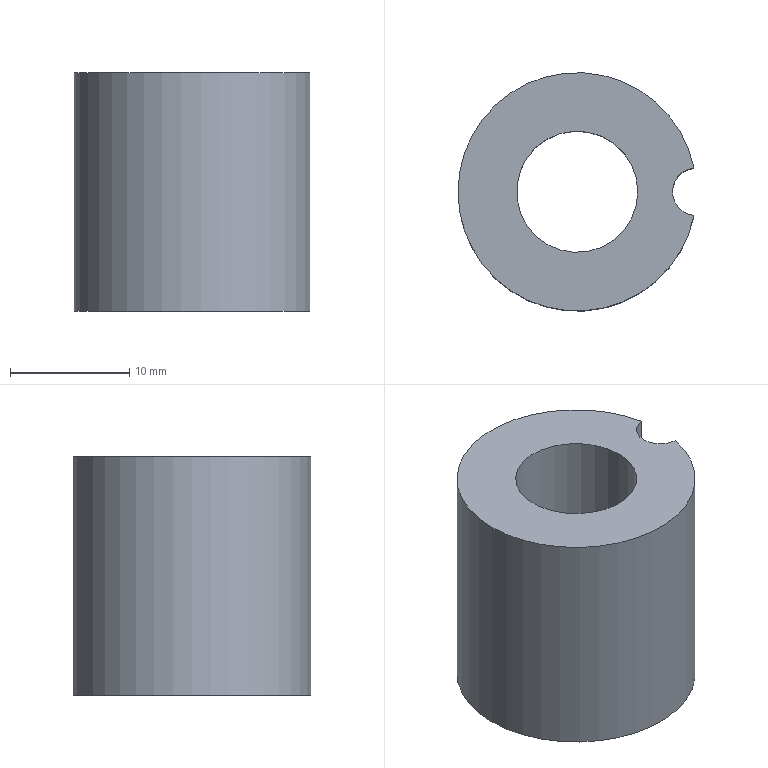Part | NX | features solid 2 | 1 solid | 7 faces | box 19.8 x 20 x 20 mm | volume 4017 mm3 | cylinder 4 | plane 3 | commonest cylinder face diameters 4 x1 10.17 x1 12.6 x1 20 x1
STEP:
#1=CARTESIAN_POINT('',(-210.056,-19.136,32.703));
#2=VERTEX_POINT('',#1);
#3=CARTESIAN_POINT('',(-210.056,-15.156,32.703));
#4=VERTEX_POINT('',#3);
#5=CARTESIAN_POINT('',(-209.856,-17.146,32.703));
#6=DIRECTION('',(0.,0.,-1.));
#7=DIRECTION('',(-1.,0.,0.));
#8=AXIS2_PLACEMENT_3D('',#5,#6,#7);
#9=CIRCLE('',#8,2.);
#10=EDGE_CURVE('',#2,#4,#9,.T.);
#11=ORIENTED_EDGE('',*,*,#10,.T.);
#12=CARTESIAN_POINT('',(-219.856,-17.146,32.703));
#13=DIRECTION('',(0.,0.,-1.));
#14=DIRECTION('',(-1.,0.,0.));
#15=AXIS2_PLACEMENT_3D('',#12,#13,#14);
#16=CIRCLE('',#15,10.);
#17=EDGE_CURVE('',#2,#4,#16,.T.);
#18=ORIENTED_EDGE('',*,*,#17,.F.);
#19=EDGE_LOOP('',(#11,#18));
#20=FACE_BOUND('',#19,.T.);
#21=CARTESIAN_POINT('',(-214.771,-17.146,32.703));
#22=VERTEX_POINT('',#21);
#23=CARTESIAN_POINT('',(-219.856,-17.146,32.703));
#24=DIRECTION('',(0.,0.,1.));
#25=DIRECTION('',(1.,0.,0.));
#26=AXIS2_PLACEMENT_3D('',#23,#24,#25);
#27=CIRCLE('',#26,5.085);
#28=EDGE_CURVE('',#22,#22,#27,.F.);
#29=ORIENTED_EDGE('',*,*,#28,.T.);
#30=EDGE_LOOP('',(#29));
#31=FACE_BOUND('',#30,.T.);
#32=CARTESIAN_POINT('',(-219.856,-17.146,32.703));
#33=DIRECTION('',(0.,0.,1.));
#34=DIRECTION('',(1.,0.,0.));
#35=AXIS2_PLACEMENT_3D('',#32,#33,#34);
#36=PLANE('',#35);
#37=ADVANCED_FACE('',(#20,#31),#36,.T.);
#38=CARTESIAN_POINT('',(-210.056,-15.156,12.703));
#39=VERTEX_POINT('',#38);
#40=CARTESIAN_POINT('',(-210.056,-19.136,12.703));
#41=VERTEX_POINT('',#40);
#42=CARTESIAN_POINT('',(-209.856,-17.146,12.703));
#43=DIRECTION('',(0.,0.,1.));
#44=DIRECTION('',(1.,0.,0.));
#45=AXIS2_PLACEMENT_3D('',#42,#43,#44);
#46=CIRCLE('',#45,2.);
#47=EDGE_CURVE('',#39,#41,#46,.T.);
#48=ORIENTED_EDGE('',*,*,#47,.T.);
#49=CARTESIAN_POINT('',(-219.856,-17.146,12.703));
#50=DIRECTION('',(0.,0.,1.));
#51=DIRECTION('',(1.,0.,0.));
#52=AXIS2_PLACEMENT_3D('',#49,#50,#51);
#53=CIRCLE('',#52,10.);
#54=EDGE_CURVE('',#39,#41,#53,.T.);
#55=ORIENTED_EDGE('',*,*,#54,.F.);
#56=EDGE_LOOP('',(#48,#55));
#57=FACE_BOUND('',#56,.T.);
#58=CARTESIAN_POINT('',(-213.556,-17.146,12.703));
#59=VERTEX_POINT('',#58);
#60=CARTESIAN_POINT('',(-219.856,-17.146,12.703));
#61=DIRECTION('',(0.,0.,1.));
#62=DIRECTION('',(1.,0.,0.));
#63=AXIS2_PLACEMENT_3D('',#60,#61,#62);
#64=CIRCLE('',#63,6.3);
#65=EDGE_CURVE('',#59,#59,#64,.T.);
#66=ORIENTED_EDGE('',*,*,#65,.T.);
#67=EDGE_LOOP('',(#66));
#68=FACE_BOUND('',#67,.T.);
#69=CARTESIAN_POINT('',(-219.856,-17.146,12.703));
#70=DIRECTION('',(0.,0.,-1.));
#71=DIRECTION('',(-1.,0.,0.));
#72=AXIS2_PLACEMENT_3D('',#69,#70,#71);
#73=PLANE('',#72);
#74=ADVANCED_FACE('',(#57,#68),#73,.T.);
#75=CARTESIAN_POINT('',(-210.056,-15.156,22.703));
#76=DIRECTION('',(0.,0.,1.));
#77=VECTOR('',#76,1000.);
#78=LINE('',#75,#77);
#79=EDGE_CURVE('',#39,#4,#78,.T.);
#80=ORIENTED_EDGE('',*,*,#79,.F.);
#81=ORIENTED_EDGE('',*,*,#54,.T.);
#82=CARTESIAN_POINT('',(-210.056,-19.136,22.703));
#83=DIRECTION('',(0.,0.,1.));
#84=VECTOR('',#83,1000.);
#85=LINE('',#82,#84);
#86=EDGE_CURVE('',#2,#41,#85,.F.);
#87=ORIENTED_EDGE('',*,*,#86,.F.);
#88=ORIENTED_EDGE('',*,*,#17,.T.);
#89=EDGE_LOOP('',(#80,#81,#87,#88));
#90=FACE_BOUND('',#89,.T.);
#91=CARTESIAN_POINT('',(-219.856,-17.146,12.703));
#92=DIRECTION('',(0.,0.,1.));
#93=DIRECTION('',(1.,0.,0.));
#94=AXIS2_PLACEMENT_3D('',#91,#92,#93);
#95=CYLINDRICAL_SURFACE('',#94,10.);
#96=ADVANCED_FACE('',(#90),#95,.T.);
#97=CARTESIAN_POINT('',(-214.771,-17.146,24.703));
#98=VERTEX_POINT('',#97);
#99=CARTESIAN_POINT('',(-219.856,-17.146,24.703));
#100=DIRECTION('',(0.,0.,1.));
#101=DIRECTION('',(1.,0.,0.));
#102=AXIS2_PLACEMENT_3D('',#99,#100,#101);
#103=CIRCLE('',#102,5.085);
#104=EDGE_CURVE('',#98,#98,#103,.T.);
#105=ORIENTED_EDGE('',*,*,#104,.T.);
#106=EDGE_LOOP('',(#105));
#107=FACE_BOUND('',#106,.T.);
#108=CARTESIAN_POINT('',(-226.156,-17.146,24.703));
#109=VERTEX_POINT('',#108);
#110=CARTESIAN_POINT('',(-219.856,-17.146,24.703));
#111=DIRECTION('',(0.,0.,-1.));
#112=DIRECTION('',(-1.,0.,0.));
#113=AXIS2_PLACEMENT_3D('',#110,#111,#112);
#114=CIRCLE('',#113,6.3);
#115=EDGE_CURVE('',#109,#109,#114,.T.);
#116=ORIENTED_EDGE('',*,*,#115,.T.);
#117=EDGE_LOOP('',(#116));
#118=FACE_BOUND('',#117,.T.);
#119=CARTESIAN_POINT('',(-219.856,-17.146,24.703));
#120=DIRECTION('',(0.,0.,1.));
#121=DIRECTION('',(1.,0.,0.));
#122=AXIS2_PLACEMENT_3D('',#119,#120,#121);
#123=PLANE('',#122);
#124=ADVANCED_FACE('',(#107,#118),#123,.F.);
#125=ORIENTED_EDGE('',*,*,#115,.F.);
#126=EDGE_LOOP('',(#125));
#127=FACE_BOUND('',#126,.T.);
#128=ORIENTED_EDGE('',*,*,#65,.F.);
#129=EDGE_LOOP('',(#128));
#130=FACE_BOUND('',#129,.T.);
#131=CARTESIAN_POINT('',(-219.856,-17.146,12.703));
#132=DIRECTION('',(0.,0.,1.));
#133=DIRECTION('',(1.,0.,0.));
#134=AXIS2_PLACEMENT_3D('',#131,#132,#133);
#135=CYLINDRICAL_SURFACE('',#134,6.3);
#136=ADVANCED_FACE('',(#127,#130),#135,.F.);
#137=ORIENTED_EDGE('',*,*,#28,.F.);
#138=EDGE_LOOP('',(#137));
#139=FACE_BOUND('',#138,.T.);
#140=ORIENTED_EDGE('',*,*,#104,.F.);
#141=EDGE_LOOP('',(#140));
#142=FACE_BOUND('',#141,.T.);
#143=CARTESIAN_POINT('',(-219.856,-17.146,24.703));
#144=DIRECTION('',(0.,0.,1.));
#145=DIRECTION('',(1.,0.,0.));
#146=AXIS2_PLACEMENT_3D('',#143,#144,#145);
#147=CYLINDRICAL_SURFACE('',#146,5.085);
#148=ADVANCED_FACE('',(#139,#142),#147,.F.);
#149=ORIENTED_EDGE('',*,*,#79,.T.);
#150=ORIENTED_EDGE('',*,*,#10,.F.);
#151=ORIENTED_EDGE('',*,*,#86,.T.);
#152=ORIENTED_EDGE('',*,*,#47,.F.);
#153=EDGE_LOOP('',(#149,#150,#151,#152));
#154=FACE_BOUND('',#153,.T.);
#155=CARTESIAN_POINT('',(-209.856,-17.146,12.703));
#156=DIRECTION('',(0.,0.,1.));
#157=DIRECTION('',(1.,0.,0.));
#158=AXIS2_PLACEMENT_3D('',#155,#156,#157);
#159=CYLINDRICAL_SURFACE('',#158,2.);
#160=ADVANCED_FACE('',(#154),#159,.F.);
#161=CLOSED_SHELL('',(#37,#74,#96,#124,#136,#148,#160));
#162=MANIFOLD_SOLID_BREP('',#161);
#163=(LENGTH_UNIT()NAMED_UNIT(*)SI_UNIT(.MILLI.,.METRE.));
#164=UNCERTAINTY_MEASURE_WITH_UNIT(LENGTH_MEASURE(0.00001),#163,'','');
#165=(NAMED_UNIT(*)PLANE_ANGLE_UNIT()SI_UNIT($,.RADIAN.));
#166=(NAMED_UNIT(*)SI_UNIT($,.STERADIAN.)SOLID_ANGLE_UNIT());
#167=(GEOMETRIC_REPRESENTATION_CONTEXT(3)GLOBAL_UNCERTAINTY_ASSIGNED_CONTEXT((#164))GLOBAL_UNIT_ASSIGNED_CONTEXT((#163,#165,#166))REPRESENTATION_CONTEXT('',''));
#168=ADVANCED_BREP_SHAPE_REPRESENTATION('',(#162),#167);